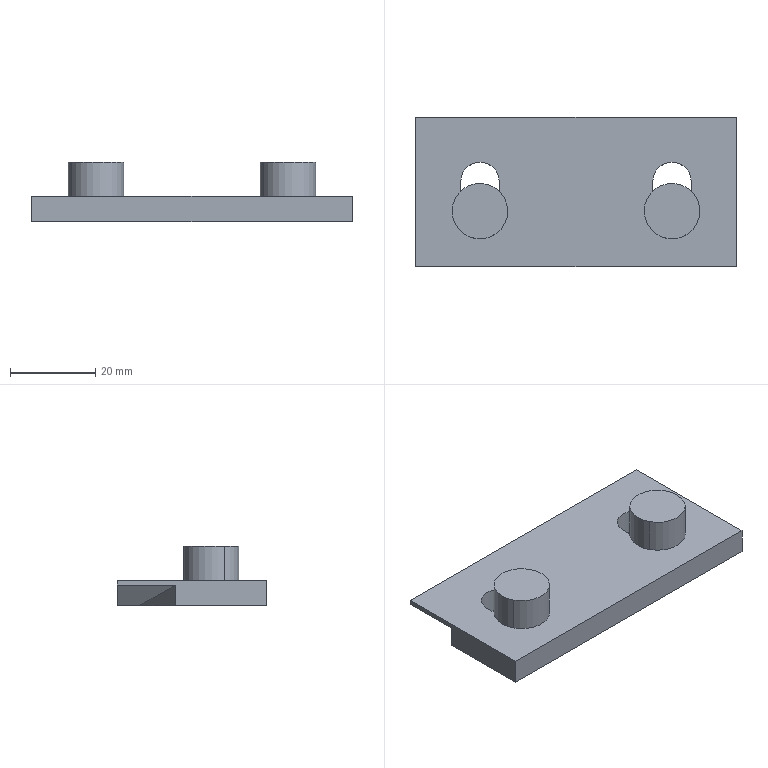Part | CATIA | 3 solids | 26 faces | box 75 x 35 x 14 mm | volume 15567 mm3 | plane 18 | cylinder 8 | commonest cylinder face diameters 9 x4 13 x4
STEP:
#1=CARTESIAN_POINT('',(-37.5,-30.,38.));
#2=VERTEX_POINT('',#1);
#3=CARTESIAN_POINT('',(-37.5,-30.,44.));
#4=VERTEX_POINT('',#3);
#5=CARTESIAN_POINT('',(-37.5,-30.,41.));
#6=DIRECTION('',(0.,0.,1.));
#7=VECTOR('',#6,1.);
#8=LINE('',#5,#7);
#9=EDGE_CURVE('',#2,#4,#8,.T.);
#10=ORIENTED_EDGE('',*,*,#9,.F.);
#11=CARTESIAN_POINT('',(37.5,-30.,38.));
#12=VERTEX_POINT('',#11);
#13=CARTESIAN_POINT('',(0.,-30.,38.));
#14=DIRECTION('',(1.,0.,0.));
#15=VECTOR('',#14,1.);
#16=LINE('',#13,#15);
#17=EDGE_CURVE('',#2,#12,#16,.T.);
#18=ORIENTED_EDGE('',*,*,#17,.T.);
#19=CARTESIAN_POINT('',(37.5,-30.,44.));
#20=VERTEX_POINT('',#19);
#21=CARTESIAN_POINT('',(37.5,-30.,41.));
#22=DIRECTION('',(0.,0.,1.));
#23=VECTOR('',#22,1.);
#24=LINE('',#21,#23);
#25=EDGE_CURVE('',#12,#20,#24,.T.);
#26=ORIENTED_EDGE('',*,*,#25,.T.);
#27=CARTESIAN_POINT('',(0.,-30.,44.));
#28=DIRECTION('',(1.,0.,0.));
#29=VECTOR('',#28,1.);
#30=LINE('',#27,#29);
#31=EDGE_CURVE('',#4,#20,#30,.T.);
#32=ORIENTED_EDGE('',*,*,#31,.F.);
#33=EDGE_LOOP('',(#10,#18,#26,#32));
#34=FACE_OUTER_BOUND('',#33,.T.);
#35=CARTESIAN_POINT('',(-37.5,-30.,38.));
#36=DIRECTION('',(0.,-1.,0.));
#37=DIRECTION('',(1.,0.,0.));
#38=AXIS2_PLACEMENT_3D('',#35,#36,#37);
#39=PLANE('',#38);
#40=ADVANCED_FACE('',(#34),#39,.T.);
#41=CARTESIAN_POINT('',(37.5,-8.66,42.874));
#42=VERTEX_POINT('',#41);
#43=CARTESIAN_POINT('',(37.5,-8.66,38.));
#44=VERTEX_POINT('',#43);
#45=CARTESIAN_POINT('',(37.5,-8.66,40.437));
#46=DIRECTION('',(0.,0.,-1.));
#47=VECTOR('',#46,1.);
#48=LINE('',#45,#47);
#49=EDGE_CURVE('',#42,#44,#48,.T.);
#50=ORIENTED_EDGE('',*,*,#49,.F.);
#51=CARTESIAN_POINT('',(37.5,5.,42.874));
#52=VERTEX_POINT('',#51);
#53=CARTESIAN_POINT('',(37.5,-1.83,42.874));
#54=DIRECTION('',(0.,1.,0.));
#55=VECTOR('',#54,1.);
#56=LINE('',#53,#55);
#57=EDGE_CURVE('',#42,#52,#56,.T.);
#58=ORIENTED_EDGE('',*,*,#57,.T.);
#59=CARTESIAN_POINT('',(37.5,5.,44.));
#60=VERTEX_POINT('',#59);
#61=CARTESIAN_POINT('',(37.5,5.,43.437));
#62=DIRECTION('',(0.,0.,1.));
#63=VECTOR('',#62,1.);
#64=LINE('',#61,#63);
#65=EDGE_CURVE('',#52,#60,#64,.T.);
#66=ORIENTED_EDGE('',*,*,#65,.T.);
#67=CARTESIAN_POINT('',(37.5,-12.5,44.));
#68=DIRECTION('',(0.,-1.,0.));
#69=VECTOR('',#68,1.);
#70=LINE('',#67,#69);
#71=EDGE_CURVE('',#20,#60,#70,.F.);
#72=ORIENTED_EDGE('',*,*,#71,.F.);
#73=ORIENTED_EDGE('',*,*,#25,.F.);
#74=CARTESIAN_POINT('',(37.5,-19.33,38.));
#75=DIRECTION('',(0.,-1.,0.));
#76=VECTOR('',#75,1.);
#77=LINE('',#74,#76);
#78=EDGE_CURVE('',#12,#44,#77,.F.);
#79=ORIENTED_EDGE('',*,*,#78,.T.);
#80=EDGE_LOOP('',(#50,#58,#66,#72,#73,#79));
#81=FACE_OUTER_BOUND('',#80,.T.);
#82=CARTESIAN_POINT('',(37.5,5.,38.));
#83=DIRECTION('',(-1.,0.,0.));
#84=DIRECTION('',(0.,-1.,0.));
#85=AXIS2_PLACEMENT_3D('',#82,#83,#84);
#86=PLANE('',#85);
#87=ADVANCED_FACE('',(#81),#86,.F.);
#88=CARTESIAN_POINT('',(-37.5,-8.66,42.874));
#89=VERTEX_POINT('',#88);
#90=CARTESIAN_POINT('',(-37.5,5.,42.874));
#91=VERTEX_POINT('',#90);
#92=CARTESIAN_POINT('',(-37.5,-1.83,42.874));
#93=DIRECTION('',(0.,1.,0.));
#94=VECTOR('',#93,1.);
#95=LINE('',#92,#94);
#96=EDGE_CURVE('',#89,#91,#95,.T.);
#97=ORIENTED_EDGE('',*,*,#96,.F.);
#98=CARTESIAN_POINT('',(-37.5,-8.66,38.));
#99=VERTEX_POINT('',#98);
#100=CARTESIAN_POINT('',(-37.5,-8.66,40.437));
#101=DIRECTION('',(0.,0.,-1.));
#102=VECTOR('',#101,1.);
#103=LINE('',#100,#102);
#104=EDGE_CURVE('',#89,#99,#103,.T.);
#105=ORIENTED_EDGE('',*,*,#104,.T.);
#106=CARTESIAN_POINT('',(-37.5,-19.33,38.));
#107=DIRECTION('',(0.,1.,0.));
#108=VECTOR('',#107,1.);
#109=LINE('',#106,#108);
#110=EDGE_CURVE('',#99,#2,#109,.F.);
#111=ORIENTED_EDGE('',*,*,#110,.T.);
#112=ORIENTED_EDGE('',*,*,#9,.T.);
#113=CARTESIAN_POINT('',(-37.5,5.,44.));
#114=VERTEX_POINT('',#113);
#115=CARTESIAN_POINT('',(-37.5,-12.5,44.));
#116=DIRECTION('',(0.,1.,0.));
#117=VECTOR('',#116,1.);
#118=LINE('',#115,#117);
#119=EDGE_CURVE('',#114,#4,#118,.F.);
#120=ORIENTED_EDGE('',*,*,#119,.F.);
#121=CARTESIAN_POINT('',(-37.5,5.,43.437));
#122=DIRECTION('',(0.,0.,1.));
#123=VECTOR('',#122,1.);
#124=LINE('',#121,#123);
#125=EDGE_CURVE('',#91,#114,#124,.T.);
#126=ORIENTED_EDGE('',*,*,#125,.F.);
#127=EDGE_LOOP('',(#97,#105,#111,#112,#120,#126));
#128=FACE_OUTER_BOUND('',#127,.T.);
#129=CARTESIAN_POINT('',(-37.5,-30.,38.));
#130=DIRECTION('',(1.,0.,0.));
#131=DIRECTION('',(0.,1.,0.));
#132=AXIS2_PLACEMENT_3D('',#129,#130,#131);
#133=PLANE('',#132);
#134=ADVANCED_FACE('',(#128),#133,.F.);
#135=CARTESIAN_POINT('',(22.5,5.,38.));
#136=VERTEX_POINT('',#135);
#137=CARTESIAN_POINT('',(-22.5,5.,38.));
#138=VERTEX_POINT('',#137);
#139=CARTESIAN_POINT('',(0.,5.,38.));
#140=DIRECTION('',(-1.,0.,0.));
#141=VECTOR('',#140,1.);
#142=LINE('',#139,#141);
#143=EDGE_CURVE('',#136,#138,#142,.T.);
#144=ORIENTED_EDGE('',*,*,#143,.T.);
#145=CARTESIAN_POINT('',(-30.,5.,40.437));
#146=DIRECTION('',(-0.9511,0.,0.309));
#147=VECTOR('',#146,1.);
#148=LINE('',#145,#147);
#149=EDGE_CURVE('',#138,#91,#148,.T.);
#150=ORIENTED_EDGE('',*,*,#149,.T.);
#151=ORIENTED_EDGE('',*,*,#125,.T.);
#152=CARTESIAN_POINT('',(0.,5.,44.));
#153=DIRECTION('',(-1.,0.,0.));
#154=VECTOR('',#153,1.);
#155=LINE('',#152,#154);
#156=EDGE_CURVE('',#60,#114,#155,.T.);
#157=ORIENTED_EDGE('',*,*,#156,.F.);
#158=ORIENTED_EDGE('',*,*,#65,.F.);
#159=CARTESIAN_POINT('',(30.,5.,40.437));
#160=DIRECTION('',(0.9511,0.,0.309));
#161=VECTOR('',#160,1.);
#162=LINE('',#159,#161);
#163=EDGE_CURVE('',#136,#52,#162,.T.);
#164=ORIENTED_EDGE('',*,*,#163,.F.);
#165=EDGE_LOOP('',(#144,#150,#151,#157,#158,#164));
#166=FACE_OUTER_BOUND('',#165,.T.);
#167=CARTESIAN_POINT('',(37.5,5.,38.));
#168=DIRECTION('',(0.,1.,0.));
#169=DIRECTION('',(-1.,0.,0.));
#170=AXIS2_PLACEMENT_3D('',#167,#168,#169);
#171=PLANE('',#170);
#172=ADVANCED_FACE('',(#166),#171,.T.);
#173=CARTESIAN_POINT('',(22.5,0.,38.));
#174=VERTEX_POINT('',#173);
#175=CARTESIAN_POINT('',(37.5,-8.66,42.874));
#176=CARTESIAN_POINT('',(22.5,0.,38.));
#177=B_SPLINE_CURVE_WITH_KNOTS('',1,(#175,#176),.UNSPECIFIED.,.F.,.U.,(2,2),(-2.999,14.994),.UNSPECIFIED.);
#178=EDGE_CURVE('',#174,#42,#177,.F.);
#179=ORIENTED_EDGE('',*,*,#178,.T.);
#180=ORIENTED_EDGE('',*,*,#49,.T.);
#181=CARTESIAN_POINT('',(35.,-7.217,38.));
#182=DIRECTION('',(0.866,-0.5,0.));
#183=VECTOR('',#182,1.);
#184=LINE('',#181,#183);
#185=EDGE_CURVE('',#174,#44,#184,.T.);
#186=ORIENTED_EDGE('',*,*,#185,.F.);
#187=EDGE_LOOP('',(#179,#180,#186));
#188=FACE_OUTER_BOUND('',#187,.T.);
#189=CARTESIAN_POINT('',(22.5,0.,38.));
#190=DIRECTION('',(0.5,0.866,0.));
#191=DIRECTION('',(0.,0.,1.));
#192=AXIS2_PLACEMENT_3D('',#189,#190,#191);
#193=PLANE('',#192);
#194=ADVANCED_FACE('',(#188),#193,.T.);
#195=ORIENTED_EDGE('',*,*,#163,.T.);
#196=ORIENTED_EDGE('',*,*,#57,.F.);
#197=ORIENTED_EDGE('',*,*,#178,.F.);
#198=CARTESIAN_POINT('',(22.5,5.,38.));
#199=DIRECTION('',(0.,-1.,0.));
#200=VECTOR('',#199,1.);
#201=LINE('',#198,#200);
#202=EDGE_CURVE('',#174,#136,#201,.F.);
#203=ORIENTED_EDGE('',*,*,#202,.T.);
#204=EDGE_LOOP('',(#195,#196,#197,#203));
#205=FACE_OUTER_BOUND('',#204,.T.);
#206=CARTESIAN_POINT('',(22.5,10.,38.));
#207=DIRECTION('',(-0.309,0.,0.9511));
#208=DIRECTION('',(0.,-1.,0.));
#209=AXIS2_PLACEMENT_3D('',#206,#207,#208);
#210=PLANE('',#209);
#211=ADVANCED_FACE('',(#205),#210,.F.);
#212=CARTESIAN_POINT('',(-22.5,0.,38.));
#213=VERTEX_POINT('',#212);
#214=CARTESIAN_POINT('',(-35.,-7.217,38.));
#215=DIRECTION('',(-0.866,-0.5,0.));
#216=VECTOR('',#215,1.);
#217=LINE('',#214,#216);
#218=EDGE_CURVE('',#213,#99,#217,.T.);
#219=ORIENTED_EDGE('',*,*,#218,.T.);
#220=ORIENTED_EDGE('',*,*,#104,.F.);
#221=CARTESIAN_POINT('',(-37.5,-8.66,42.874));
#222=CARTESIAN_POINT('',(-22.5,0.,38.));
#223=B_SPLINE_CURVE_WITH_KNOTS('',1,(#221,#222),.UNSPECIFIED.,.F.,.U.,(2,2),(-2.999,14.994),.UNSPECIFIED.);
#224=EDGE_CURVE('',#213,#89,#223,.F.);
#225=ORIENTED_EDGE('',*,*,#224,.F.);
#226=EDGE_LOOP('',(#219,#220,#225));
#227=FACE_OUTER_BOUND('',#226,.T.);
#228=CARTESIAN_POINT('',(-22.5,0.,38.));
#229=DIRECTION('',(0.5,-0.866,0.));
#230=DIRECTION('',(0.,0.,1.));
#231=AXIS2_PLACEMENT_3D('',#228,#229,#230);
#232=PLANE('',#231);
#233=ADVANCED_FACE('',(#227),#232,.F.);
#234=CARTESIAN_POINT('',(-22.5,5.,38.));
#235=DIRECTION('',(0.,-1.,0.));
#236=VECTOR('',#235,1.);
#237=LINE('',#234,#236);
#238=EDGE_CURVE('',#213,#138,#237,.F.);
#239=ORIENTED_EDGE('',*,*,#238,.F.);
#240=ORIENTED_EDGE('',*,*,#224,.T.);
#241=ORIENTED_EDGE('',*,*,#96,.T.);
#242=ORIENTED_EDGE('',*,*,#149,.F.);
#243=EDGE_LOOP('',(#239,#240,#241,#242));
#244=FACE_OUTER_BOUND('',#243,.T.);
#245=CARTESIAN_POINT('',(-22.5,10.,38.));
#246=DIRECTION('',(-0.309,0.,-0.9511));
#247=DIRECTION('',(0.,-1.,0.));
#248=AXIS2_PLACEMENT_3D('',#245,#246,#247);
#249=PLANE('',#248);
#250=ADVANCED_FACE('',(#244),#249,.T.);
#251=ORIENTED_EDGE('',*,*,#143,.F.);
#252=ORIENTED_EDGE('',*,*,#202,.F.);
#253=ORIENTED_EDGE('',*,*,#185,.T.);
#254=ORIENTED_EDGE('',*,*,#78,.F.);
#255=ORIENTED_EDGE('',*,*,#17,.F.);
#256=ORIENTED_EDGE('',*,*,#110,.F.);
#257=ORIENTED_EDGE('',*,*,#218,.F.);
#258=ORIENTED_EDGE('',*,*,#238,.T.);
#259=EDGE_LOOP('',(#251,#252,#253,#254,#255,#256,#257,#258));
#260=FACE_OUTER_BOUND('',#259,.T.);
#261=CARTESIAN_POINT('',(-18.,-10.,38.));
#262=VERTEX_POINT('',#261);
#263=CARTESIAN_POINT('',(-18.,-17.,38.));
#264=VERTEX_POINT('',#263);
#265=CARTESIAN_POINT('',(-18.,-13.5,38.));
#266=DIRECTION('',(0.,-1.,0.));
#267=VECTOR('',#266,1.);
#268=LINE('',#265,#267);
#269=EDGE_CURVE('',#262,#264,#268,.T.);
#270=ORIENTED_EDGE('',*,*,#269,.F.);
#271=CARTESIAN_POINT('',(-27.,-10.,38.));
#272=VERTEX_POINT('',#271);
#273=CARTESIAN_POINT('',(-22.5,-10.,38.));
#274=DIRECTION('',(0.,0.,1.));
#275=AXIS2_PLACEMENT_3D('',#273,#274,$);
#276=CIRCLE('',#275,4.5);
#277=EDGE_CURVE('',#262,#272,#276,.T.);
#278=ORIENTED_EDGE('',*,*,#277,.T.);
#279=CARTESIAN_POINT('',(-27.,-17.,38.));
#280=VERTEX_POINT('',#279);
#281=CARTESIAN_POINT('',(-27.,-13.5,38.));
#282=DIRECTION('',(0.,-1.,0.));
#283=VECTOR('',#282,1.);
#284=LINE('',#281,#283);
#285=EDGE_CURVE('',#272,#280,#284,.T.);
#286=ORIENTED_EDGE('',*,*,#285,.T.);
#287=CARTESIAN_POINT('',(-22.5,-17.,38.));
#288=DIRECTION('',(0.,0.,1.));
#289=AXIS2_PLACEMENT_3D('',#287,#288,$);
#290=CIRCLE('',#289,4.5);
#291=EDGE_CURVE('',#280,#264,#290,.T.);
#292=ORIENTED_EDGE('',*,*,#291,.T.);
#293=EDGE_LOOP('',(#270,#278,#286,#292));
#294=FACE_BOUND('',#293,.T.);
#295=CARTESIAN_POINT('',(27.,-10.,38.));
#296=VERTEX_POINT('',#295);
#297=CARTESIAN_POINT('',(18.,-10.,38.));
#298=VERTEX_POINT('',#297);
#299=CARTESIAN_POINT('',(22.5,-10.,38.));
#300=DIRECTION('',(0.,0.,1.));
#301=AXIS2_PLACEMENT_3D('',#299,#300,$);
#302=CIRCLE('',#301,4.5);
#303=EDGE_CURVE('',#296,#298,#302,.T.);
#304=ORIENTED_EDGE('',*,*,#303,.T.);
#305=CARTESIAN_POINT('',(18.,-17.,38.));
#306=VERTEX_POINT('',#305);
#307=CARTESIAN_POINT('',(18.,-13.5,38.));
#308=DIRECTION('',(0.,-1.,0.));
#309=VECTOR('',#308,1.);
#310=LINE('',#307,#309);
#311=EDGE_CURVE('',#298,#306,#310,.T.);
#312=ORIENTED_EDGE('',*,*,#311,.T.);
#313=CARTESIAN_POINT('',(27.,-17.,38.));
#314=VERTEX_POINT('',#313);
#315=CARTESIAN_POINT('',(22.5,-17.,38.));
#316=DIRECTION('',(0.,0.,1.));
#317=AXIS2_PLACEMENT_3D('',#315,#316,$);
#318=CIRCLE('',#317,4.5);
#319=EDGE_CURVE('',#306,#314,#318,.T.);
#320=ORIENTED_EDGE('',*,*,#319,.T.);
#321=CARTESIAN_POINT('',(27.,-13.5,38.));
#322=DIRECTION('',(0.,-1.,0.));
#323=VECTOR('',#322,1.);
#324=LINE('',#321,#323);
#325=EDGE_CURVE('',#296,#314,#324,.T.);
#326=ORIENTED_EDGE('',*,*,#325,.F.);
#327=EDGE_LOOP('',(#304,#312,#320,#326));
#328=FACE_BOUND('',#327,.T.);
#329=CARTESIAN_POINT('',(0.,0.,38.));
#330=DIRECTION('',(0.,0.,1.));
#331=DIRECTION('',(1.,0.,0.));
#332=AXIS2_PLACEMENT_3D('',#329,#330,#331);
#333=PLANE('',#332);
#334=ADVANCED_FACE('',(#260,#294,#328),#333,.F.);
#335=ORIENTED_EDGE('',*,*,#156,.T.);
#336=ORIENTED_EDGE('',*,*,#119,.T.);
#337=ORIENTED_EDGE('',*,*,#31,.T.);
#338=ORIENTED_EDGE('',*,*,#71,.T.);
#339=EDGE_LOOP('',(#335,#336,#337,#338));
#340=FACE_OUTER_BOUND('',#339,.T.);
#341=CARTESIAN_POINT('',(-18.,-17.,44.));
#342=VERTEX_POINT('',#341);
#343=CARTESIAN_POINT('',(-18.,-10.,44.));
#344=VERTEX_POINT('',#343);
#345=CARTESIAN_POINT('',(-18.,-13.5,44.));
#346=DIRECTION('',(0.,-1.,0.));
#347=VECTOR('',#346,1.);
#348=LINE('',#345,#347);
#349=EDGE_CURVE('',#342,#344,#348,.F.);
#350=ORIENTED_EDGE('',*,*,#349,.F.);
#351=CARTESIAN_POINT('',(-27.,-17.,44.));
#352=VERTEX_POINT('',#351);
#353=CARTESIAN_POINT('',(-22.5,-17.,44.));
#354=DIRECTION('',(0.,0.,1.));
#355=AXIS2_PLACEMENT_3D('',#353,#354,$);
#356=CIRCLE('',#355,4.5);
#357=EDGE_CURVE('',#352,#342,#356,.T.);
#358=ORIENTED_EDGE('',*,*,#357,.F.);
#359=CARTESIAN_POINT('',(-27.,-10.,44.));
#360=VERTEX_POINT('',#359);
#361=CARTESIAN_POINT('',(-27.,-13.5,44.));
#362=DIRECTION('',(0.,-1.,0.));
#363=VECTOR('',#362,1.);
#364=LINE('',#361,#363);
#365=EDGE_CURVE('',#360,#352,#364,.T.);
#366=ORIENTED_EDGE('',*,*,#365,.F.);
#367=CARTESIAN_POINT('',(-22.5,-10.,44.));
#368=DIRECTION('',(0.,0.,1.));
#369=AXIS2_PLACEMENT_3D('',#367,#368,$);
#370=CIRCLE('',#369,4.5);
#371=EDGE_CURVE('',#344,#360,#370,.T.);
#372=ORIENTED_EDGE('',*,*,#371,.F.);
#373=EDGE_LOOP('',(#350,#358,#366,#372));
#374=FACE_BOUND('',#373,.T.);
#375=CARTESIAN_POINT('',(27.,-10.,44.));
#376=VERTEX_POINT('',#375);
#377=CARTESIAN_POINT('',(18.,-10.,44.));
#378=VERTEX_POINT('',#377);
#379=CARTESIAN_POINT('',(22.5,-10.,44.));
#380=DIRECTION('',(0.,0.,1.));
#381=AXIS2_PLACEMENT_3D('',#379,#380,$);
#382=CIRCLE('',#381,4.5);
#383=EDGE_CURVE('',#376,#378,#382,.T.);
#384=ORIENTED_EDGE('',*,*,#383,.F.);
#385=CARTESIAN_POINT('',(27.,-17.,44.));
#386=VERTEX_POINT('',#385);
#387=CARTESIAN_POINT('',(27.,-13.5,44.));
#388=DIRECTION('',(0.,-1.,0.));
#389=VECTOR('',#388,1.);
#390=LINE('',#387,#389);
#391=EDGE_CURVE('',#386,#376,#390,.F.);
#392=ORIENTED_EDGE('',*,*,#391,.F.);
#393=CARTESIAN_POINT('',(18.,-17.,44.));
#394=VERTEX_POINT('',#393);
#395=CARTESIAN_POINT('',(22.5,-17.,44.));
#396=DIRECTION('',(0.,0.,1.));
#397=AXIS2_PLACEMENT_3D('',#395,#396,$);
#398=CIRCLE('',#397,4.5);
#399=EDGE_CURVE('',#394,#386,#398,.T.);
#400=ORIENTED_EDGE('',*,*,#399,.F.);
#401=CARTESIAN_POINT('',(18.,-13.5,44.));
#402=DIRECTION('',(0.,-1.,0.));
#403=VECTOR('',#402,1.);
#404=LINE('',#401,#403);
#405=EDGE_CURVE('',#378,#394,#404,.T.);
#406=ORIENTED_EDGE('',*,*,#405,.F.);
#407=EDGE_LOOP('',(#384,#392,#400,#406));
#408=FACE_BOUND('',#407,.T.);
#409=CARTESIAN_POINT('',(0.,0.,44.));
#410=DIRECTION('',(0.,0.,1.));
#411=DIRECTION('',(1.,0.,0.));
#412=AXIS2_PLACEMENT_3D('',#409,#410,#411);
#413=PLANE('',#412);
#414=ADVANCED_FACE('',(#340,#374,#408),#413,.T.);
#415=ORIENTED_EDGE('',*,*,#303,.F.);
#416=CARTESIAN_POINT('',(27.,-10.,34.));
#417=DIRECTION('',(0.,0.,1.));
#418=VECTOR('',#417,1.);
#419=LINE('',#416,#418);
#420=EDGE_CURVE('',#376,#296,#419,.F.);
#421=ORIENTED_EDGE('',*,*,#420,.F.);
#422=ORIENTED_EDGE('',*,*,#383,.T.);
#423=CARTESIAN_POINT('',(18.,-10.,34.));
#424=DIRECTION('',(0.,0.,1.));
#425=VECTOR('',#424,1.);
#426=LINE('',#423,#425);
#427=EDGE_CURVE('',#378,#298,#426,.F.);
#428=ORIENTED_EDGE('',*,*,#427,.T.);
#429=EDGE_LOOP('',(#415,#421,#422,#428));
#430=FACE_OUTER_BOUND('',#429,.T.);
#431=CARTESIAN_POINT('',(22.5,-10.,34.));
#432=DIRECTION('',(0.,0.,1.));
#433=DIRECTION('',(1.,0.,0.));
#434=AXIS2_PLACEMENT_3D('',#431,#432,#433);
#435=CYLINDRICAL_SURFACE('',#434,4.5);
#436=ADVANCED_FACE('',(#430),#435,.F.);
#437=ORIENTED_EDGE('',*,*,#427,.F.);
#438=ORIENTED_EDGE('',*,*,#405,.T.);
#439=CARTESIAN_POINT('',(18.,-17.,41.));
#440=DIRECTION('',(0.,0.,-1.));
#441=VECTOR('',#440,1.);
#442=LINE('',#439,#441);
#443=EDGE_CURVE('',#394,#306,#442,.T.);
#444=ORIENTED_EDGE('',*,*,#443,.T.);
#445=ORIENTED_EDGE('',*,*,#311,.F.);
#446=EDGE_LOOP('',(#437,#438,#444,#445));
#447=FACE_OUTER_BOUND('',#446,.T.);
#448=CARTESIAN_POINT('',(18.,-10.,44.));
#449=DIRECTION('',(1.,0.,0.));
#450=DIRECTION('',(0.,-1.,0.));
#451=AXIS2_PLACEMENT_3D('',#448,#449,#450);
#452=PLANE('',#451);
#453=ADVANCED_FACE('',(#447),#452,.T.);
#454=ORIENTED_EDGE('',*,*,#325,.T.);
#455=CARTESIAN_POINT('',(27.,-17.,41.));
#456=DIRECTION('',(0.,0.,-1.));
#457=VECTOR('',#456,1.);
#458=LINE('',#455,#457);
#459=EDGE_CURVE('',#386,#314,#458,.T.);
#460=ORIENTED_EDGE('',*,*,#459,.F.);
#461=ORIENTED_EDGE('',*,*,#391,.T.);
#462=ORIENTED_EDGE('',*,*,#420,.T.);
#463=EDGE_LOOP('',(#454,#460,#461,#462));
#464=FACE_OUTER_BOUND('',#463,.T.);
#465=CARTESIAN_POINT('',(27.,-10.,44.));
#466=DIRECTION('',(1.,0.,0.));
#467=DIRECTION('',(0.,-1.,0.));
#468=AXIS2_PLACEMENT_3D('',#465,#466,#467);
#469=PLANE('',#468);
#470=ADVANCED_FACE('',(#464),#469,.F.);
#471=ORIENTED_EDGE('',*,*,#319,.F.);
#472=ORIENTED_EDGE('',*,*,#443,.F.);
#473=ORIENTED_EDGE('',*,*,#399,.T.);
#474=ORIENTED_EDGE('',*,*,#459,.T.);
#475=EDGE_LOOP('',(#471,#472,#473,#474));
#476=FACE_OUTER_BOUND('',#475,.T.);
#477=CARTESIAN_POINT('',(22.5,-17.,34.));
#478=DIRECTION('',(0.,0.,1.));
#479=DIRECTION('',(-1.,0.,0.));
#480=AXIS2_PLACEMENT_3D('',#477,#478,#479);
#481=CYLINDRICAL_SURFACE('',#480,4.5);
#482=ADVANCED_FACE('',(#476),#481,.F.);
#483=ORIENTED_EDGE('',*,*,#269,.T.);
#484=CARTESIAN_POINT('',(-18.,-17.,41.));
#485=DIRECTION('',(0.,0.,-1.));
#486=VECTOR('',#485,1.);
#487=LINE('',#484,#486);
#488=EDGE_CURVE('',#342,#264,#487,.T.);
#489=ORIENTED_EDGE('',*,*,#488,.F.);
#490=ORIENTED_EDGE('',*,*,#349,.T.);
#491=CARTESIAN_POINT('',(-18.,-10.,41.));
#492=DIRECTION('',(0.,0.,-1.));
#493=VECTOR('',#492,1.);
#494=LINE('',#491,#493);
#495=EDGE_CURVE('',#344,#262,#494,.T.);
#496=ORIENTED_EDGE('',*,*,#495,.T.);
#497=EDGE_LOOP('',(#483,#489,#490,#496));
#498=FACE_OUTER_BOUND('',#497,.T.);
#499=CARTESIAN_POINT('',(-18.,-10.,44.));
#500=DIRECTION('',(1.,0.,0.));
#501=DIRECTION('',(0.,-1.,0.));
#502=AXIS2_PLACEMENT_3D('',#499,#500,#501);
#503=PLANE('',#502);
#504=ADVANCED_FACE('',(#498),#503,.F.);
#505=ORIENTED_EDGE('',*,*,#277,.F.);
#506=ORIENTED_EDGE('',*,*,#495,.F.);
#507=ORIENTED_EDGE('',*,*,#371,.T.);
#508=CARTESIAN_POINT('',(-27.,-10.,34.));
#509=DIRECTION('',(0.,0.,1.));
#510=VECTOR('',#509,1.);
#511=LINE('',#508,#510);
#512=EDGE_CURVE('',#360,#272,#511,.F.);
#513=ORIENTED_EDGE('',*,*,#512,.T.);
#514=EDGE_LOOP('',(#505,#506,#507,#513));
#515=FACE_OUTER_BOUND('',#514,.T.);
#516=CARTESIAN_POINT('',(-22.5,-10.,34.));
#517=DIRECTION('',(0.,0.,1.));
#518=DIRECTION('',(1.,0.,0.));
#519=AXIS2_PLACEMENT_3D('',#516,#517,#518);
#520=CYLINDRICAL_SURFACE('',#519,4.5);
#521=ADVANCED_FACE('',(#515),#520,.F.);
#522=ORIENTED_EDGE('',*,*,#291,.F.);
#523=CARTESIAN_POINT('',(-27.,-17.,34.));
#524=DIRECTION('',(0.,0.,1.));
#525=VECTOR('',#524,1.);
#526=LINE('',#523,#525);
#527=EDGE_CURVE('',#352,#280,#526,.F.);
#528=ORIENTED_EDGE('',*,*,#527,.F.);
#529=ORIENTED_EDGE('',*,*,#357,.T.);
#530=ORIENTED_EDGE('',*,*,#488,.T.);
#531=EDGE_LOOP('',(#522,#528,#529,#530));
#532=FACE_OUTER_BOUND('',#531,.T.);
#533=CARTESIAN_POINT('',(-22.5,-17.,34.));
#534=DIRECTION('',(0.,0.,1.));
#535=DIRECTION('',(-1.,0.,0.));
#536=AXIS2_PLACEMENT_3D('',#533,#534,#535);
#537=CYLINDRICAL_SURFACE('',#536,4.5);
#538=ADVANCED_FACE('',(#532),#537,.F.);
#539=ORIENTED_EDGE('',*,*,#512,.F.);
#540=ORIENTED_EDGE('',*,*,#365,.T.);
#541=ORIENTED_EDGE('',*,*,#527,.T.);
#542=ORIENTED_EDGE('',*,*,#285,.F.);
#543=EDGE_LOOP('',(#539,#540,#541,#542));
#544=FACE_OUTER_BOUND('',#543,.T.);
#545=CARTESIAN_POINT('',(-27.,-10.,44.));
#546=DIRECTION('',(1.,0.,0.));
#547=DIRECTION('',(0.,-1.,0.));
#548=AXIS2_PLACEMENT_3D('',#545,#546,#547);
#549=PLANE('',#548);
#550=ADVANCED_FACE('',(#544),#549,.T.);
#551=CLOSED_SHELL('',(#40,#87,#134,#172,#194,#211,#233,#250,#334,#414,#436,#453,#470,#482,#504,#521,#538,#550));
#552=MANIFOLD_SOLID_BREP('',#551);
#553=CARTESIAN_POINT('',(-16.796,-13.884,52.));
#554=VERTEX_POINT('',#553);
#555=CARTESIAN_POINT('',(-28.204,-20.116,52.));
#556=VERTEX_POINT('',#555);
#557=CARTESIAN_POINT('',(-22.5,-17.,52.));
#558=DIRECTION('',(0.,0.,1.));
#559=AXIS2_PLACEMENT_3D('',#557,#558,$);
#560=CIRCLE('',#559,6.5);
#561=EDGE_CURVE('',#554,#556,#560,.T.);
#562=ORIENTED_EDGE('',*,*,#561,.T.);
#563=CARTESIAN_POINT('',(-22.5,-17.,52.));
#564=DIRECTION('',(0.,0.,1.));
#565=AXIS2_PLACEMENT_3D('',#563,#564,$);
#566=CIRCLE('',#565,6.5);
#567=EDGE_CURVE('',#556,#554,#566,.T.);
#568=ORIENTED_EDGE('',*,*,#567,.T.);
#569=EDGE_LOOP('',(#562,#568));
#570=FACE_OUTER_BOUND('',#569,.T.);
#571=CARTESIAN_POINT('',(-22.5,-17.,52.));
#572=DIRECTION('',(0.,0.,1.));
#573=DIRECTION('',(1.,0.,0.));
#574=AXIS2_PLACEMENT_3D('',#571,#572,#573);
#575=PLANE('',#574);
#576=ADVANCED_FACE('',(#570),#575,.T.);
#577=CARTESIAN_POINT('',(-28.204,-20.116,44.));
#578=VERTEX_POINT('',#577);
#579=CARTESIAN_POINT('',(-28.204,-20.116,47.8));
#580=DIRECTION('',(0.,0.,1.));
#581=VECTOR('',#580,1.);
#582=LINE('',#579,#581);
#583=EDGE_CURVE('',#556,#578,#582,.F.);
#584=ORIENTED_EDGE('',*,*,#583,.F.);
#585=ORIENTED_EDGE('',*,*,#561,.F.);
#586=CARTESIAN_POINT('',(-16.796,-13.884,44.));
#587=VERTEX_POINT('',#586);
#588=CARTESIAN_POINT('',(-16.796,-13.884,47.8));
#589=DIRECTION('',(0.,0.,1.));
#590=VECTOR('',#589,1.);
#591=LINE('',#588,#590);
#592=EDGE_CURVE('',#554,#587,#591,.F.);
#593=ORIENTED_EDGE('',*,*,#592,.T.);
#594=CARTESIAN_POINT('',(-22.5,-17.,44.));
#595=DIRECTION('',(0.,0.,1.));
#596=AXIS2_PLACEMENT_3D('',#594,#595,$);
#597=CIRCLE('',#596,6.5);
#598=EDGE_CURVE('',#587,#578,#597,.T.);
#599=ORIENTED_EDGE('',*,*,#598,.T.);
#600=EDGE_LOOP('',(#584,#585,#593,#599));
#601=FACE_OUTER_BOUND('',#600,.T.);
#602=CARTESIAN_POINT('',(-22.5,-17.,44.1));
#603=DIRECTION('',(0.,0.,1.));
#604=DIRECTION('',(0.8776,0.4794,0.));
#605=AXIS2_PLACEMENT_3D('',#602,#603,#604);
#606=CYLINDRICAL_SURFACE('',#605,6.5);
#607=ADVANCED_FACE('',(#601),#606,.T.);
#608=ORIENTED_EDGE('',*,*,#592,.F.);
#609=ORIENTED_EDGE('',*,*,#567,.F.);
#610=ORIENTED_EDGE('',*,*,#583,.T.);
#611=CARTESIAN_POINT('',(-22.5,-17.,44.));
#612=DIRECTION('',(0.,0.,1.));
#613=AXIS2_PLACEMENT_3D('',#611,#612,$);
#614=CIRCLE('',#613,6.5);
#615=EDGE_CURVE('',#578,#587,#614,.T.);
#616=ORIENTED_EDGE('',*,*,#615,.T.);
#617=EDGE_LOOP('',(#608,#609,#610,#616));
#618=FACE_OUTER_BOUND('',#617,.T.);
#619=ADVANCED_FACE('',(#618),#606,.T.);
#620=ORIENTED_EDGE('',*,*,#598,.F.);
#621=ORIENTED_EDGE('',*,*,#615,.F.);
#622=EDGE_LOOP('',(#620,#621));
#623=FACE_OUTER_BOUND('',#622,.T.);
#624=ADVANCED_FACE('',(#623),#413,.F.);
#625=CLOSED_SHELL('',(#576,#607,#619,#624));
#626=MANIFOLD_SOLID_BREP('',#625);
#627=CARTESIAN_POINT('',(28.204,-13.884,52.));
#628=VERTEX_POINT('',#627);
#629=CARTESIAN_POINT('',(16.796,-20.116,52.));
#630=VERTEX_POINT('',#629);
#631=CARTESIAN_POINT('',(22.5,-17.,52.));
#632=DIRECTION('',(0.,0.,1.));
#633=AXIS2_PLACEMENT_3D('',#631,#632,$);
#634=CIRCLE('',#633,6.5);
#635=EDGE_CURVE('',#628,#630,#634,.T.);
#636=ORIENTED_EDGE('',*,*,#635,.T.);
#637=CARTESIAN_POINT('',(22.5,-17.,52.));
#638=DIRECTION('',(0.,0.,1.));
#639=AXIS2_PLACEMENT_3D('',#637,#638,$);
#640=CIRCLE('',#639,6.5);
#641=EDGE_CURVE('',#630,#628,#640,.T.);
#642=ORIENTED_EDGE('',*,*,#641,.T.);
#643=EDGE_LOOP('',(#636,#642));
#644=FACE_OUTER_BOUND('',#643,.T.);
#645=ADVANCED_FACE('',(#644),#575,.T.);
#646=CARTESIAN_POINT('',(16.796,-20.116,44.));
#647=VERTEX_POINT('',#646);
#648=CARTESIAN_POINT('',(16.796,-20.116,47.8));
#649=DIRECTION('',(0.,0.,1.));
#650=VECTOR('',#649,1.);
#651=LINE('',#648,#650);
#652=EDGE_CURVE('',#630,#647,#651,.F.);
#653=ORIENTED_EDGE('',*,*,#652,.F.);
#654=ORIENTED_EDGE('',*,*,#635,.F.);
#655=CARTESIAN_POINT('',(28.204,-13.884,44.));
#656=VERTEX_POINT('',#655);
#657=CARTESIAN_POINT('',(28.204,-13.884,47.8));
#658=DIRECTION('',(0.,0.,1.));
#659=VECTOR('',#658,1.);
#660=LINE('',#657,#659);
#661=EDGE_CURVE('',#628,#656,#660,.F.);
#662=ORIENTED_EDGE('',*,*,#661,.T.);
#663=CARTESIAN_POINT('',(22.5,-17.,44.));
#664=DIRECTION('',(0.,0.,1.));
#665=AXIS2_PLACEMENT_3D('',#663,#664,$);
#666=CIRCLE('',#665,6.5);
#667=EDGE_CURVE('',#656,#647,#666,.T.);
#668=ORIENTED_EDGE('',*,*,#667,.T.);
#669=EDGE_LOOP('',(#653,#654,#662,#668));
#670=FACE_OUTER_BOUND('',#669,.T.);
#671=CARTESIAN_POINT('',(22.5,-17.,44.1));
#672=DIRECTION('',(0.,0.,1.));
#673=DIRECTION('',(0.8776,0.4794,0.));
#674=AXIS2_PLACEMENT_3D('',#671,#672,#673);
#675=CYLINDRICAL_SURFACE('',#674,6.5);
#676=ADVANCED_FACE('',(#670),#675,.T.);
#677=ORIENTED_EDGE('',*,*,#661,.F.);
#678=ORIENTED_EDGE('',*,*,#641,.F.);
#679=ORIENTED_EDGE('',*,*,#652,.T.);
#680=CARTESIAN_POINT('',(22.5,-17.,44.));
#681=DIRECTION('',(0.,0.,1.));
#682=AXIS2_PLACEMENT_3D('',#680,#681,$);
#683=CIRCLE('',#682,6.5);
#684=EDGE_CURVE('',#647,#656,#683,.T.);
#685=ORIENTED_EDGE('',*,*,#684,.T.);
#686=EDGE_LOOP('',(#677,#678,#679,#685));
#687=FACE_OUTER_BOUND('',#686,.T.);
#688=ADVANCED_FACE('',(#687),#675,.T.);
#689=ORIENTED_EDGE('',*,*,#667,.F.);
#690=ORIENTED_EDGE('',*,*,#684,.F.);
#691=EDGE_LOOP('',(#689,#690));
#692=FACE_OUTER_BOUND('',#691,.T.);
#693=ADVANCED_FACE('',(#692),#413,.F.);
#694=CLOSED_SHELL('',(#645,#676,#688,#693));
#695=MANIFOLD_SOLID_BREP('',#694);
#696=(LENGTH_UNIT()NAMED_UNIT(*)SI_UNIT(.MILLI.,.METRE.));
#697=UNCERTAINTY_MEASURE_WITH_UNIT(LENGTH_MEASURE(0.005),#696,'','');
#698=(NAMED_UNIT(*)PLANE_ANGLE_UNIT()SI_UNIT($,.RADIAN.));
#699=(NAMED_UNIT(*)SI_UNIT($,.STERADIAN.)SOLID_ANGLE_UNIT());
#700=(GEOMETRIC_REPRESENTATION_CONTEXT(3)GLOBAL_UNCERTAINTY_ASSIGNED_CONTEXT((#697))GLOBAL_UNIT_ASSIGNED_CONTEXT((#696,#698,#699))REPRESENTATION_CONTEXT('',''));
#701=ADVANCED_BREP_SHAPE_REPRESENTATION('',(#552,#626,#695),#700);